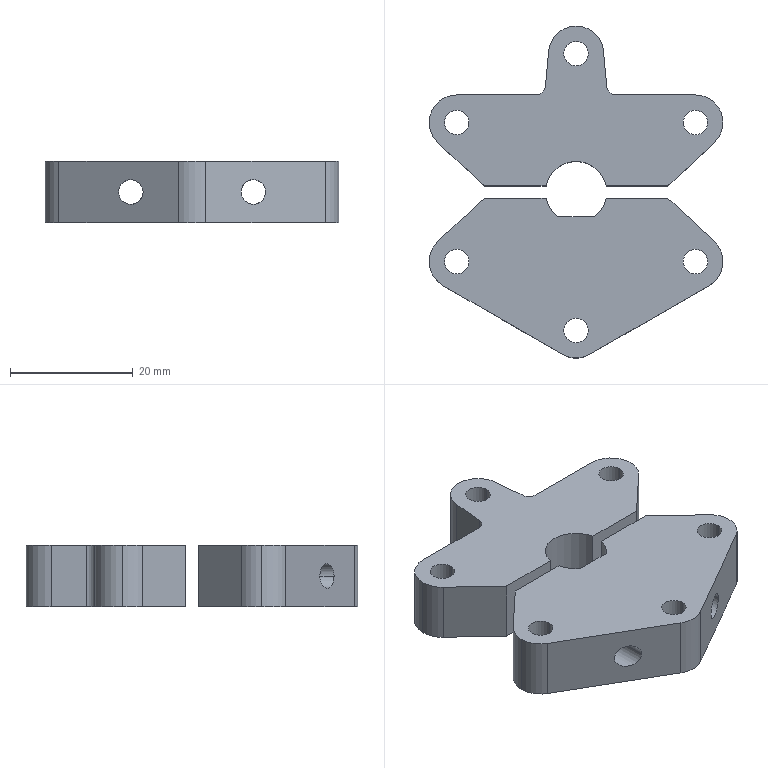Part | SolidWorks | features BaseBody 2 | 2 solids | 52 faces | box 47.971 x 54.2 x 10 mm | volume 13527 mm3 | cylinder 33 | plane 19 | commonest cylinder face diameters 4 x16 9 x8 5.2 x4 10 x3 3 x2